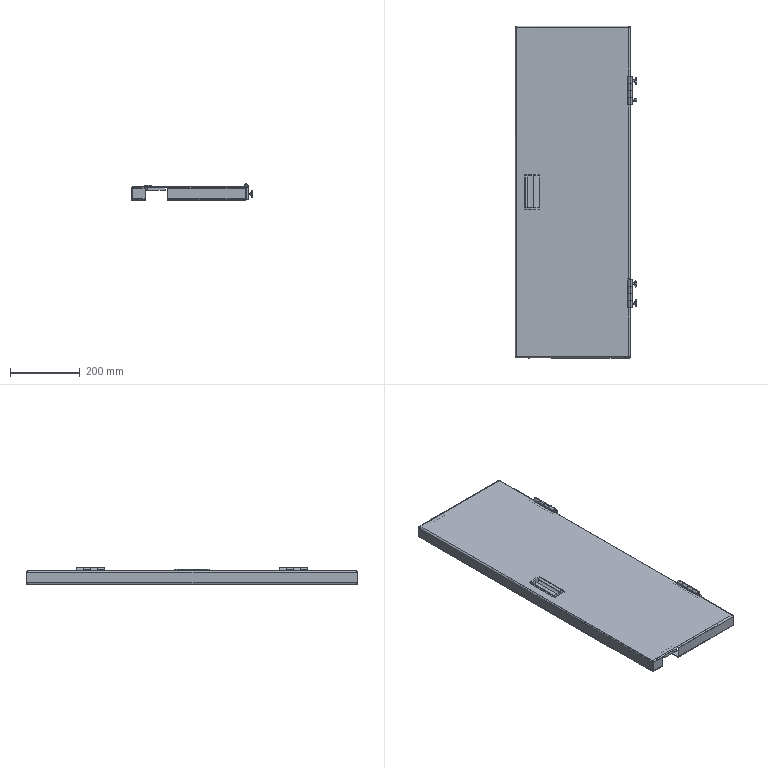Part | SolidWorks | features ReferencePattern 5, LocalLPattern 1 | 25 solids | 676 faces | box 349.5 x 954 x 47.25 mm | volume 1020587 mm3 | plane 365 | cylinder 183 | cone 88 | spline 40 | commonest cylinder face diameters 8 x30 5 x24 11.5 x24 7 x20 10 x20 4 x16